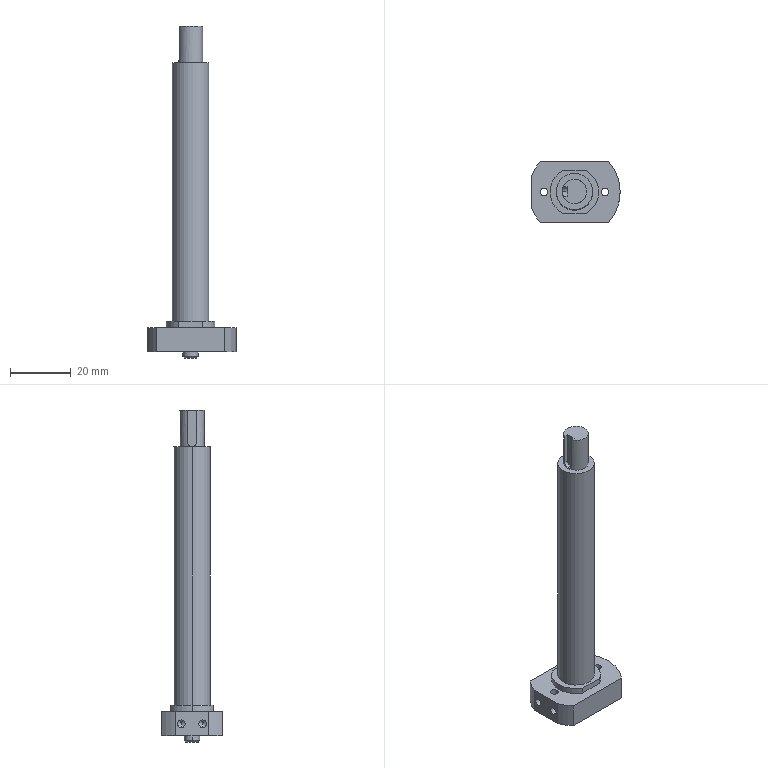Part | STEP file | 06-01-02 rotary shaft | 1 solid | 42 faces | box 29 x 20 x 109 mm | volume 14786 mm3 | cylinder 22 | plane 14 | cone 6 | commonest cylinder face diameters 2.5 x8 16 x3 30 x3 3 x2 5 x2 8 x2
STEP:
#1=CARTESIAN_POINT('',(-6.5,-3.5,2.75));
#2=VERTEX_POINT('',#1);
#3=CARTESIAN_POINT('',(-6.5,-3.5,5.25));
#4=VERTEX_POINT('',#3);
#5=CARTESIAN_POINT('',(-6.5,-3.5,4.));
#6=DIRECTION('',(-1.,0.,0.));
#7=DIRECTION('',(0.,0.,1.));
#8=AXIS2_PLACEMENT_3D('',#5,#6,#7);
#9=CIRCLE('',#8,1.25);
#10=EDGE_CURVE('',#2,#4,#9,.T.);
#11=ORIENTED_EDGE('',*,*,#10,.F.);
#12=CARTESIAN_POINT('',(-14.,-3.5,2.75));
#13=VERTEX_POINT('',#12);
#14=CARTESIAN_POINT('',(-14.,-3.5,2.75));
#15=DIRECTION('',(-1.,0.,0.));
#16=VECTOR('',#15,1000.);
#17=LINE('',#14,#16);
#18=EDGE_CURVE('',#2,#13,#17,.T.);
#19=ORIENTED_EDGE('',*,*,#18,.T.);
#20=CARTESIAN_POINT('',(-14.,-3.5,5.25));
#21=VERTEX_POINT('',#20);
#22=CARTESIAN_POINT('',(-14.,-3.5,4.));
#23=DIRECTION('',(-1.,0.,0.));
#24=DIRECTION('',(0.,0.,1.));
#25=AXIS2_PLACEMENT_3D('',#22,#23,#24);
#26=CIRCLE('',#25,1.25);
#27=EDGE_CURVE('',#13,#21,#26,.T.);
#28=ORIENTED_EDGE('',*,*,#27,.T.);
#29=CARTESIAN_POINT('',(-14.,-3.5,5.25));
#30=DIRECTION('',(-1.,0.,0.));
#31=VECTOR('',#30,1000.);
#32=LINE('',#29,#31);
#33=EDGE_CURVE('',#4,#21,#32,.T.);
#34=ORIENTED_EDGE('',*,*,#33,.F.);
#35=EDGE_LOOP('',(#11,#19,#28,#34));
#36=FACE_OUTER_BOUND('',#35,.T.);
#37=CARTESIAN_POINT('',(-14.,-3.5,4.));
#38=DIRECTION('',(-1.,0.,0.));
#39=DIRECTION('',(0.,0.,1.));
#40=AXIS2_PLACEMENT_3D('',#37,#38,#39);
#41=CYLINDRICAL_SURFACE('',#40,1.25);
#42=ADVANCED_FACE('',(#36),#41,.F.);
#43=CARTESIAN_POINT('',(-5.749,-3.5,4.));
#44=VERTEX_POINT('',#43);
#45=CARTESIAN_POINT('',(-6.5,-3.5,5.25));
#46=DIRECTION('',(-0.515,0.,0.8572));
#47=VECTOR('',#46,1000.);
#48=LINE('',#45,#47);
#49=EDGE_CURVE('',#44,#4,#48,.T.);
#50=ORIENTED_EDGE('',*,*,#49,.F.);
#51=CARTESIAN_POINT('',(-6.5,-3.5,2.75));
#52=DIRECTION('',(-0.515,0.,-0.8572));
#53=VECTOR('',#52,1000.);
#54=LINE('',#51,#53);
#55=EDGE_CURVE('',#44,#2,#54,.T.);
#56=ORIENTED_EDGE('',*,*,#55,.T.);
#57=ORIENTED_EDGE('',*,*,#10,.T.);
#58=EDGE_LOOP('',(#50,#56,#57));
#59=FACE_OUTER_BOUND('',#58,.T.);
#60=CARTESIAN_POINT('',(-6.5,-3.5,4.));
#61=DIRECTION('',(-1.,0.,0.));
#62=DIRECTION('',(0.,0.,1.));
#63=AXIS2_PLACEMENT_3D('',#60,#61,#62);
#64=CONICAL_SURFACE('',#63,1.25,1.03);
#65=ADVANCED_FACE('',(#59),#64,.F.);
#66=CARTESIAN_POINT('',(-6.5,3.5,2.75));
#67=VERTEX_POINT('',#66);
#68=CARTESIAN_POINT('',(-6.5,3.5,5.25));
#69=VERTEX_POINT('',#68);
#70=CARTESIAN_POINT('',(-6.5,3.5,4.));
#71=DIRECTION('',(-1.,0.,0.));
#72=DIRECTION('',(0.,0.,1.));
#73=AXIS2_PLACEMENT_3D('',#70,#71,#72);
#74=CIRCLE('',#73,1.25);
#75=EDGE_CURVE('',#67,#69,#74,.T.);
#76=ORIENTED_EDGE('',*,*,#75,.F.);
#77=CARTESIAN_POINT('',(-14.,3.5,2.75));
#78=VERTEX_POINT('',#77);
#79=CARTESIAN_POINT('',(-14.,3.5,2.75));
#80=DIRECTION('',(-1.,0.,0.));
#81=VECTOR('',#80,1000.);
#82=LINE('',#79,#81);
#83=EDGE_CURVE('',#67,#78,#82,.T.);
#84=ORIENTED_EDGE('',*,*,#83,.T.);
#85=CARTESIAN_POINT('',(-14.,3.5,5.25));
#86=VERTEX_POINT('',#85);
#87=CARTESIAN_POINT('',(-14.,3.5,4.));
#88=DIRECTION('',(-1.,0.,0.));
#89=DIRECTION('',(0.,0.,1.));
#90=AXIS2_PLACEMENT_3D('',#87,#88,#89);
#91=CIRCLE('',#90,1.25);
#92=EDGE_CURVE('',#78,#86,#91,.T.);
#93=ORIENTED_EDGE('',*,*,#92,.T.);
#94=CARTESIAN_POINT('',(-14.,3.5,5.25));
#95=DIRECTION('',(-1.,0.,0.));
#96=VECTOR('',#95,1000.);
#97=LINE('',#94,#96);
#98=EDGE_CURVE('',#69,#86,#97,.T.);
#99=ORIENTED_EDGE('',*,*,#98,.F.);
#100=EDGE_LOOP('',(#76,#84,#93,#99));
#101=FACE_OUTER_BOUND('',#100,.T.);
#102=CARTESIAN_POINT('',(-14.,3.5,4.));
#103=DIRECTION('',(-1.,0.,0.));
#104=DIRECTION('',(0.,0.,1.));
#105=AXIS2_PLACEMENT_3D('',#102,#103,#104);
#106=CYLINDRICAL_SURFACE('',#105,1.25);
#107=ADVANCED_FACE('',(#101),#106,.F.);
#108=CARTESIAN_POINT('',(-5.749,3.5,4.));
#109=VERTEX_POINT('',#108);
#110=CARTESIAN_POINT('',(-6.5,3.5,5.25));
#111=DIRECTION('',(-0.515,0.,0.8572));
#112=VECTOR('',#111,1000.);
#113=LINE('',#110,#112);
#114=EDGE_CURVE('',#109,#69,#113,.T.);
#115=ORIENTED_EDGE('',*,*,#114,.F.);
#116=CARTESIAN_POINT('',(-6.5,3.5,2.75));
#117=DIRECTION('',(-0.515,0.,-0.8572));
#118=VECTOR('',#117,1000.);
#119=LINE('',#116,#118);
#120=EDGE_CURVE('',#109,#67,#119,.T.);
#121=ORIENTED_EDGE('',*,*,#120,.T.);
#122=ORIENTED_EDGE('',*,*,#75,.T.);
#123=EDGE_LOOP('',(#115,#121,#122));
#124=FACE_OUTER_BOUND('',#123,.T.);
#125=CARTESIAN_POINT('',(-6.5,3.5,4.));
#126=DIRECTION('',(-1.,0.,0.));
#127=DIRECTION('',(0.,0.,1.));
#128=AXIS2_PLACEMENT_3D('',#125,#126,#127);
#129=CONICAL_SURFACE('',#128,1.25,1.03);
#130=ADVANCED_FACE('',(#124),#129,.F.);
#131=CARTESIAN_POINT('',(-2.,0.,-2.));
#132=VERTEX_POINT('',#131);
#133=CARTESIAN_POINT('',(2.,0.,-2.));
#134=VERTEX_POINT('',#133);
#135=CARTESIAN_POINT('',(0.,0.,-2.));
#136=DIRECTION('',(0.,0.,-1.));
#137=DIRECTION('',(-1.,0.,0.));
#138=AXIS2_PLACEMENT_3D('',#135,#136,#137);
#139=CIRCLE('',#138,2.);
#140=EDGE_CURVE('',#132,#134,#139,.T.);
#141=ORIENTED_EDGE('',*,*,#140,.F.);
#142=CARTESIAN_POINT('',(-2.5,0.,-1.5));
#143=VERTEX_POINT('',#142);
#144=CARTESIAN_POINT('',(-2.,0.,-2.));
#145=DIRECTION('',(-0.7071,0.,0.7071));
#146=VECTOR('',#145,1000.);
#147=LINE('',#144,#146);
#148=EDGE_CURVE('',#132,#143,#147,.T.);
#149=ORIENTED_EDGE('',*,*,#148,.T.);
#150=CARTESIAN_POINT('',(2.5,0.,-1.5));
#151=VERTEX_POINT('',#150);
#152=CARTESIAN_POINT('',(0.,0.,-1.5));
#153=DIRECTION('',(0.,0.,1.));
#154=DIRECTION('',(-1.,0.,0.));
#155=AXIS2_PLACEMENT_3D('',#152,#153,#154);
#156=CIRCLE('',#155,2.5);
#157=EDGE_CURVE('',#151,#143,#156,.T.);
#158=ORIENTED_EDGE('',*,*,#157,.F.);
#159=CARTESIAN_POINT('',(2.,0.,-2.));
#160=DIRECTION('',(0.7071,0.,0.7071));
#161=VECTOR('',#160,1000.);
#162=LINE('',#159,#161);
#163=EDGE_CURVE('',#134,#151,#162,.T.);
#164=ORIENTED_EDGE('',*,*,#163,.F.);
#165=EDGE_LOOP('',(#141,#149,#158,#164));
#166=FACE_OUTER_BOUND('',#165,.T.);
#167=CARTESIAN_POINT('',(0.,0.,-2.));
#168=DIRECTION('',(0.,0.,1.));
#169=DIRECTION('',(1.,0.,0.));
#170=AXIS2_PLACEMENT_3D('',#167,#168,#169);
#171=CONICAL_SURFACE('',#170,2.,0.7854);
#172=ADVANCED_FACE('',(#166),#171,.T.);
#173=CARTESIAN_POINT('',(8.75,0.,8.));
#174=VERTEX_POINT('',#173);
#175=CARTESIAN_POINT('',(11.25,0.,8.));
#176=VERTEX_POINT('',#175);
#177=CARTESIAN_POINT('',(10.,0.,8.));
#178=DIRECTION('',(0.,0.,1.));
#179=DIRECTION('',(1.,0.,0.));
#180=AXIS2_PLACEMENT_3D('',#177,#178,#179);
#181=CIRCLE('',#180,1.25);
#182=EDGE_CURVE('',#174,#176,#181,.T.);
#183=ORIENTED_EDGE('',*,*,#182,.T.);
#184=CARTESIAN_POINT('',(11.25,0.,0.));
#185=VERTEX_POINT('',#184);
#186=CARTESIAN_POINT('',(11.25,0.,0.));
#187=DIRECTION('',(0.,0.,-1.));
#188=VECTOR('',#187,1000.);
#189=LINE('',#186,#188);
#190=EDGE_CURVE('',#176,#185,#189,.T.);
#191=ORIENTED_EDGE('',*,*,#190,.T.);
#192=CARTESIAN_POINT('',(8.75,0.,0.));
#193=VERTEX_POINT('',#192);
#194=CARTESIAN_POINT('',(10.,0.,0.));
#195=DIRECTION('',(0.,0.,-1.));
#196=DIRECTION('',(-1.,0.,0.));
#197=AXIS2_PLACEMENT_3D('',#194,#195,#196);
#198=CIRCLE('',#197,1.25);
#199=EDGE_CURVE('',#185,#193,#198,.T.);
#200=ORIENTED_EDGE('',*,*,#199,.T.);
#201=CARTESIAN_POINT('',(8.75,0.,0.));
#202=DIRECTION('',(0.,0.,-1.));
#203=VECTOR('',#202,1000.);
#204=LINE('',#201,#203);
#205=EDGE_CURVE('',#174,#193,#204,.T.);
#206=ORIENTED_EDGE('',*,*,#205,.F.);
#207=EDGE_LOOP('',(#183,#191,#200,#206));
#208=FACE_OUTER_BOUND('',#207,.T.);
#209=CARTESIAN_POINT('',(10.,0.,0.));
#210=DIRECTION('',(0.,0.,-1.));
#211=DIRECTION('',(-1.,0.,0.));
#212=AXIS2_PLACEMENT_3D('',#209,#210,#211);
#213=CYLINDRICAL_SURFACE('',#212,1.25);
#214=ADVANCED_FACE('',(#208),#213,.F.);
#215=CARTESIAN_POINT('',(-11.25,0.,8.));
#216=VERTEX_POINT('',#215);
#217=CARTESIAN_POINT('',(-8.75,0.,8.));
#218=VERTEX_POINT('',#217);
#219=CARTESIAN_POINT('',(-10.,0.,8.));
#220=DIRECTION('',(0.,0.,1.));
#221=DIRECTION('',(1.,0.,0.));
#222=AXIS2_PLACEMENT_3D('',#219,#220,#221);
#223=CIRCLE('',#222,1.25);
#224=EDGE_CURVE('',#216,#218,#223,.T.);
#225=ORIENTED_EDGE('',*,*,#224,.T.);
#226=CARTESIAN_POINT('',(-8.75,0.,0.));
#227=VERTEX_POINT('',#226);
#228=CARTESIAN_POINT('',(-8.75,0.,0.));
#229=DIRECTION('',(0.,0.,-1.));
#230=VECTOR('',#229,1000.);
#231=LINE('',#228,#230);
#232=EDGE_CURVE('',#218,#227,#231,.T.);
#233=ORIENTED_EDGE('',*,*,#232,.T.);
#234=CARTESIAN_POINT('',(-11.25,0.,0.));
#235=VERTEX_POINT('',#234);
#236=CARTESIAN_POINT('',(-10.,0.,0.));
#237=DIRECTION('',(0.,0.,-1.));
#238=DIRECTION('',(-1.,0.,0.));
#239=AXIS2_PLACEMENT_3D('',#236,#237,#238);
#240=CIRCLE('',#239,1.25);
#241=EDGE_CURVE('',#227,#235,#240,.T.);
#242=ORIENTED_EDGE('',*,*,#241,.T.);
#243=CARTESIAN_POINT('',(-11.25,0.,0.));
#244=DIRECTION('',(0.,0.,-1.));
#245=VECTOR('',#244,1000.);
#246=LINE('',#243,#245);
#247=EDGE_CURVE('',#216,#235,#246,.T.);
#248=ORIENTED_EDGE('',*,*,#247,.F.);
#249=EDGE_LOOP('',(#225,#233,#242,#248));
#250=FACE_OUTER_BOUND('',#249,.T.);
#251=CARTESIAN_POINT('',(-10.,0.,0.));
#252=DIRECTION('',(0.,0.,-1.));
#253=DIRECTION('',(-1.,0.,0.));
#254=AXIS2_PLACEMENT_3D('',#251,#252,#253);
#255=CYLINDRICAL_SURFACE('',#254,1.25);
#256=ADVANCED_FACE('',(#250),#255,.F.);
#257=CARTESIAN_POINT('',(4.,0.,107.));
#258=VERTEX_POINT('',#257);
#259=CARTESIAN_POINT('',(-3.708,1.5,107.));
#260=VERTEX_POINT('',#259);
#261=CARTESIAN_POINT('',(0.,0.,107.));
#262=DIRECTION('',(0.,0.,1.));
#263=DIRECTION('',(1.,0.,0.));
#264=AXIS2_PLACEMENT_3D('',#261,#262,#263);
#265=CIRCLE('',#264,4.);
#266=EDGE_CURVE('',#258,#260,#265,.T.);
#267=ORIENTED_EDGE('',*,*,#266,.F.);
#268=CARTESIAN_POINT('',(4.,0.,95.));
#269=VERTEX_POINT('',#268);
#270=CARTESIAN_POINT('',(4.,0.,107.));
#271=DIRECTION('',(0.,0.,-1.));
#272=VECTOR('',#271,1000.);
#273=LINE('',#270,#272);
#274=EDGE_CURVE('',#258,#269,#273,.T.);
#275=ORIENTED_EDGE('',*,*,#274,.T.);
#276=CARTESIAN_POINT('',(-4.,0.,95.));
#277=VERTEX_POINT('',#276);
#278=CARTESIAN_POINT('',(0.,0.,95.));
#279=DIRECTION('',(0.,0.,1.));
#280=DIRECTION('',(1.,0.,0.));
#281=AXIS2_PLACEMENT_3D('',#278,#279,#280);
#282=CIRCLE('',#281,4.);
#283=EDGE_CURVE('',#269,#277,#282,.T.);
#284=ORIENTED_EDGE('',*,*,#283,.T.);
#285=CARTESIAN_POINT('',(-3.708,1.5,96.5));
#286=VERTEX_POINT('',#285);
#287=CARTESIAN_POINT('',(-4.,0.,95.));
#288=CARTESIAN_POINT('',(-4.,0.1,95.));
#289=CARTESIAN_POINT('',(-3.996,0.1982,95.01));
#290=CARTESIAN_POINT('',(-3.982,0.3911,95.049));
#291=CARTESIAN_POINT('',(-3.971,0.4868,95.078));
#292=CARTESIAN_POINT('',(-3.932,0.7587,95.191));
#293=CARTESIAN_POINT('',(-3.894,0.9238,95.302));
#294=CARTESIAN_POINT('',(-3.819,1.198,95.576));
#295=CARTESIAN_POINT('',(-3.781,1.309,95.742));
#296=CARTESIAN_POINT('',(-3.725,1.459,96.102));
#297=CARTESIAN_POINT('',(-3.708,1.5,96.3));
#298=CARTESIAN_POINT('',(-3.708,1.5,96.5));
#299=B_SPLINE_CURVE_WITH_KNOTS('',3,(#287,#288,#289,#290,#291,#292,#293,#294,#295,#296,#297,#298),.UNSPECIFIED.,.F.,.F.,(4,2,2,2,2,4),(0.,0.0002957,0.0005913,0.001183,0.001774,0.002365),.UNSPECIFIED.);
#300=EDGE_CURVE('',#277,#286,#299,.T.);
#301=ORIENTED_EDGE('',*,*,#300,.T.);
#302=CARTESIAN_POINT('',(-3.708,1.5,107.));
#303=DIRECTION('',(0.,0.,1.));
#304=VECTOR('',#303,1000.);
#305=LINE('',#302,#304);
#306=EDGE_CURVE('',#286,#260,#305,.T.);
#307=ORIENTED_EDGE('',*,*,#306,.T.);
#308=EDGE_LOOP('',(#267,#275,#284,#301,#307));
#309=FACE_OUTER_BOUND('',#308,.T.);
#310=CARTESIAN_POINT('',(0.,0.,107.));
#311=DIRECTION('',(0.,0.,-1.));
#312=DIRECTION('',(-1.,0.,0.));
#313=AXIS2_PLACEMENT_3D('',#310,#311,#312);
#314=CYLINDRICAL_SURFACE('',#313,4.);
#315=ADVANCED_FACE('',(#309),#314,.T.);
#316=CARTESIAN_POINT('',(6.,0.,95.));
#317=VERTEX_POINT('',#316);
#318=CARTESIAN_POINT('',(-6.,0.,95.));
#319=VERTEX_POINT('',#318);
#320=CARTESIAN_POINT('',(0.,0.,95.));
#321=DIRECTION('',(0.,0.,1.));
#322=DIRECTION('',(1.,0.,0.));
#323=AXIS2_PLACEMENT_3D('',#320,#321,#322);
#324=CIRCLE('',#323,6.);
#325=EDGE_CURVE('',#317,#319,#324,.T.);
#326=ORIENTED_EDGE('',*,*,#325,.F.);
#327=CARTESIAN_POINT('',(6.,0.,10.));
#328=VERTEX_POINT('',#327);
#329=CARTESIAN_POINT('',(6.,0.,95.));
#330=DIRECTION('',(0.,0.,-1.));
#331=VECTOR('',#330,1000.);
#332=LINE('',#329,#331);
#333=EDGE_CURVE('',#317,#328,#332,.T.);
#334=ORIENTED_EDGE('',*,*,#333,.T.);
#335=CARTESIAN_POINT('',(-6.,0.,10.));
#336=VERTEX_POINT('',#335);
#337=CARTESIAN_POINT('',(0.,0.,10.));
#338=DIRECTION('',(0.,0.,1.));
#339=DIRECTION('',(1.,0.,0.));
#340=AXIS2_PLACEMENT_3D('',#337,#338,#339);
#341=CIRCLE('',#340,6.);
#342=EDGE_CURVE('',#328,#336,#341,.T.);
#343=ORIENTED_EDGE('',*,*,#342,.T.);
#344=CARTESIAN_POINT('',(-6.,0.,95.));
#345=DIRECTION('',(0.,0.,-1.));
#346=VECTOR('',#345,1000.);
#347=LINE('',#344,#346);
#348=EDGE_CURVE('',#319,#336,#347,.T.);
#349=ORIENTED_EDGE('',*,*,#348,.F.);
#350=EDGE_LOOP('',(#326,#334,#343,#349));
#351=FACE_OUTER_BOUND('',#350,.T.);
#352=CARTESIAN_POINT('',(0.,0.,95.));
#353=DIRECTION('',(0.,0.,-1.));
#354=DIRECTION('',(-1.,0.,0.));
#355=AXIS2_PLACEMENT_3D('',#352,#353,#354);
#356=CYLINDRICAL_SURFACE('',#355,6.);
#357=ADVANCED_FACE('',(#351),#356,.T.);
#358=CARTESIAN_POINT('',(-8.,0.,10.));
#359=VERTEX_POINT('',#358);
#360=CARTESIAN_POINT('',(-3.873,-7.,10.));
#361=VERTEX_POINT('',#360);
#362=CARTESIAN_POINT('',(0.,0.,10.));
#363=DIRECTION('',(0.,0.,1.));
#364=DIRECTION('',(1.,0.,0.));
#365=AXIS2_PLACEMENT_3D('',#362,#363,#364);
#366=CIRCLE('',#365,8.);
#367=EDGE_CURVE('',#359,#361,#366,.T.);
#368=ORIENTED_EDGE('',*,*,#367,.F.);
#369=CARTESIAN_POINT('',(-8.,0.,8.));
#370=VERTEX_POINT('',#369);
#371=CARTESIAN_POINT('',(-8.,0.,10.));
#372=DIRECTION('',(0.,0.,-1.));
#373=VECTOR('',#372,1000.);
#374=LINE('',#371,#373);
#375=EDGE_CURVE('',#359,#370,#374,.T.);
#376=ORIENTED_EDGE('',*,*,#375,.T.);
#377=CARTESIAN_POINT('',(-3.873,-7.,8.));
#378=VERTEX_POINT('',#377);
#379=CARTESIAN_POINT('',(0.,0.,8.));
#380=DIRECTION('',(0.,0.,1.));
#381=DIRECTION('',(1.,0.,0.));
#382=AXIS2_PLACEMENT_3D('',#379,#380,#381);
#383=CIRCLE('',#382,8.);
#384=EDGE_CURVE('',#370,#378,#383,.T.);
#385=ORIENTED_EDGE('',*,*,#384,.T.);
#386=CARTESIAN_POINT('',(-3.873,-7.,10.));
#387=DIRECTION('',(0.,0.,-1.));
#388=VECTOR('',#387,1000.);
#389=LINE('',#386,#388);
#390=EDGE_CURVE('',#361,#378,#389,.T.);
#391=ORIENTED_EDGE('',*,*,#390,.F.);
#392=EDGE_LOOP('',(#368,#376,#385,#391));
#393=FACE_OUTER_BOUND('',#392,.T.);
#394=CARTESIAN_POINT('',(0.,0.,10.));
#395=DIRECTION('',(0.,0.,-1.));
#396=DIRECTION('',(-1.,0.,0.));
#397=AXIS2_PLACEMENT_3D('',#394,#395,#396);
#398=CYLINDRICAL_SURFACE('',#397,8.);
#399=ADVANCED_FACE('',(#393),#398,.T.);
#400=ORIENTED_EDGE('',*,*,#157,.T.);
#401=CARTESIAN_POINT('',(-2.5,0.,0.));
#402=VERTEX_POINT('',#401);
#403=CARTESIAN_POINT('',(-2.5,0.,-2.));
#404=DIRECTION('',(0.,0.,1.));
#405=VECTOR('',#404,1000.);
#406=LINE('',#403,#405);
#407=EDGE_CURVE('',#143,#402,#406,.T.);
#408=ORIENTED_EDGE('',*,*,#407,.T.);
#409=CARTESIAN_POINT('',(2.5,0.,0.));
#410=VERTEX_POINT('',#409);
#411=CARTESIAN_POINT('',(0.,0.,0.));
#412=DIRECTION('',(0.,0.,-1.));
#413=DIRECTION('',(1.,0.,0.));
#414=AXIS2_PLACEMENT_3D('',#411,#412,#413);
#415=CIRCLE('',#414,2.5);
#416=EDGE_CURVE('',#402,#410,#415,.T.);
#417=ORIENTED_EDGE('',*,*,#416,.T.);
#418=CARTESIAN_POINT('',(2.5,0.,-2.));
#419=DIRECTION('',(0.,0.,1.));
#420=VECTOR('',#419,1000.);
#421=LINE('',#418,#420);
#422=EDGE_CURVE('',#151,#410,#421,.T.);
#423=ORIENTED_EDGE('',*,*,#422,.F.);
#424=EDGE_LOOP('',(#400,#408,#417,#423));
#425=FACE_OUTER_BOUND('',#424,.T.);
#426=CARTESIAN_POINT('',(0.,0.,-2.));
#427=DIRECTION('',(0.,0.,1.));
#428=DIRECTION('',(1.,0.,0.));
#429=AXIS2_PLACEMENT_3D('',#426,#427,#428);
#430=CYLINDRICAL_SURFACE('',#429,2.5);
#431=ADVANCED_FACE('',(#425),#430,.T.);
#432=CARTESIAN_POINT('',(-14.,-5.385,0.));
#433=VERTEX_POINT('',#432);
#434=CARTESIAN_POINT('',(-14.,-5.385,8.));
#435=VERTEX_POINT('',#434);
#436=CARTESIAN_POINT('',(-14.,-5.385,17.));
#437=DIRECTION('',(0.,0.,1.));
#438=VECTOR('',#437,1000.);
#439=LINE('',#436,#438);
#440=EDGE_CURVE('',#433,#435,#439,.T.);
#441=ORIENTED_EDGE('',*,*,#440,.F.);
#442=CARTESIAN_POINT('',(-11.18,-10.,0.));
#443=VERTEX_POINT('',#442);
#444=CARTESIAN_POINT('',(0.,0.,0.));
#445=DIRECTION('',(0.,0.,-1.));
#446=DIRECTION('',(-1.,0.,0.));
#447=AXIS2_PLACEMENT_3D('',#444,#445,#446);
#448=CIRCLE('',#447,15.);
#449=EDGE_CURVE('',#443,#433,#448,.T.);
#450=ORIENTED_EDGE('',*,*,#449,.F.);
#451=CARTESIAN_POINT('',(-11.18,-10.,8.));
#452=VERTEX_POINT('',#451);
#453=CARTESIAN_POINT('',(-11.18,-10.,17.));
#454=DIRECTION('',(0.,0.,1.));
#455=VECTOR('',#454,1000.);
#456=LINE('',#453,#455);
#457=EDGE_CURVE('',#443,#452,#456,.T.);
#458=ORIENTED_EDGE('',*,*,#457,.T.);
#459=CARTESIAN_POINT('',(0.,0.,8.));
#460=DIRECTION('',(0.,0.,1.));
#461=DIRECTION('',(1.,0.,0.));
#462=AXIS2_PLACEMENT_3D('',#459,#460,#461);
#463=CIRCLE('',#462,15.);
#464=EDGE_CURVE('',#435,#452,#463,.T.);
#465=ORIENTED_EDGE('',*,*,#464,.F.);
#466=EDGE_LOOP('',(#441,#450,#458,#465));
#467=FACE_OUTER_BOUND('',#466,.T.);
#468=CARTESIAN_POINT('',(0.,0.,17.));
#469=DIRECTION('',(0.,0.,-1.));
#470=DIRECTION('',(-1.,0.,0.));
#471=AXIS2_PLACEMENT_3D('',#468,#469,#470);
#472=CYLINDRICAL_SURFACE('',#471,15.);
#473=ADVANCED_FACE('',(#467),#472,.T.);
#474=CARTESIAN_POINT('',(0.,0.,95.));
#475=DIRECTION('',(0.,0.,1.));
#476=DIRECTION('',(1.,0.,0.));
#477=AXIS2_PLACEMENT_3D('',#474,#475,#476);
#478=CIRCLE('',#477,4.);
#479=EDGE_CURVE('',#277,#269,#478,.T.);
#480=ORIENTED_EDGE('',*,*,#479,.F.);
#481=ORIENTED_EDGE('',*,*,#283,.F.);
#482=EDGE_LOOP('',(#480,#481));
#483=FACE_BOUND('',#482,.T.);
#484=CARTESIAN_POINT('',(0.,0.,95.));
#485=DIRECTION('',(0.,0.,1.));
#486=DIRECTION('',(1.,0.,0.));
#487=AXIS2_PLACEMENT_3D('',#484,#485,#486);
#488=CIRCLE('',#487,6.);
#489=EDGE_CURVE('',#319,#317,#488,.T.);
#490=ORIENTED_EDGE('',*,*,#489,.T.);
#491=ORIENTED_EDGE('',*,*,#325,.T.);
#492=EDGE_LOOP('',(#490,#491));
#493=FACE_OUTER_BOUND('',#492,.T.);
#494=CARTESIAN_POINT('',(0.,0.,95.));
#495=DIRECTION('',(0.,0.,1.));
#496=DIRECTION('',(1.,0.,0.));
#497=AXIS2_PLACEMENT_3D('',#494,#495,#496);
#498=PLANE('',#497);
#499=ADVANCED_FACE('',(#483,#493),#498,.T.);
#500=CARTESIAN_POINT('',(3.873,-7.,10.));
#501=VERTEX_POINT('',#500);
#502=CARTESIAN_POINT('',(3.873,7.,10.));
#503=VERTEX_POINT('',#502);
#504=CARTESIAN_POINT('',(0.,0.,10.));
#505=DIRECTION('',(0.,0.,1.));
#506=DIRECTION('',(1.,0.,0.));
#507=AXIS2_PLACEMENT_3D('',#504,#505,#506);
#508=CIRCLE('',#507,8.);
#509=EDGE_CURVE('',#501,#503,#508,.T.);
#510=ORIENTED_EDGE('',*,*,#509,.T.);
#511=CARTESIAN_POINT('',(-3.873,7.,10.));
#512=VERTEX_POINT('',#511);
#513=CARTESIAN_POINT('',(-3.873,7.,10.));
#514=DIRECTION('',(-1.,0.,0.));
#515=VECTOR('',#514,1000.);
#516=LINE('',#513,#515);
#517=EDGE_CURVE('',#503,#512,#516,.T.);
#518=ORIENTED_EDGE('',*,*,#517,.T.);
#519=CARTESIAN_POINT('',(0.,0.,10.));
#520=DIRECTION('',(0.,0.,1.));
#521=DIRECTION('',(1.,0.,0.));
#522=AXIS2_PLACEMENT_3D('',#519,#520,#521);
#523=CIRCLE('',#522,8.);
#524=EDGE_CURVE('',#512,#359,#523,.T.);
#525=ORIENTED_EDGE('',*,*,#524,.T.);
#526=ORIENTED_EDGE('',*,*,#367,.T.);
#527=CARTESIAN_POINT('',(-3.873,-7.,10.));
#528=DIRECTION('',(1.,0.,0.));
#529=VECTOR('',#528,1000.);
#530=LINE('',#527,#529);
#531=EDGE_CURVE('',#361,#501,#530,.T.);
#532=ORIENTED_EDGE('',*,*,#531,.T.);
#533=EDGE_LOOP('',(#510,#518,#525,#526,#532));
#534=FACE_OUTER_BOUND('',#533,.T.);
#535=CARTESIAN_POINT('',(0.,0.,10.));
#536=DIRECTION('',(0.,0.,1.));
#537=DIRECTION('',(1.,0.,0.));
#538=AXIS2_PLACEMENT_3D('',#535,#536,#537);
#539=CIRCLE('',#538,6.);
#540=EDGE_CURVE('',#336,#328,#539,.T.);
#541=ORIENTED_EDGE('',*,*,#540,.F.);
#542=ORIENTED_EDGE('',*,*,#342,.F.);
#543=EDGE_LOOP('',(#541,#542));
#544=FACE_BOUND('',#543,.T.);
#545=CARTESIAN_POINT('',(0.,0.,10.));
#546=DIRECTION('',(0.,0.,1.));
#547=DIRECTION('',(1.,0.,0.));
#548=AXIS2_PLACEMENT_3D('',#545,#546,#547);
#549=PLANE('',#548);
#550=ADVANCED_FACE('',(#534,#544),#549,.T.);
#551=CARTESIAN_POINT('',(-14.,5.385,8.));
#552=VERTEX_POINT('',#551);
#553=CARTESIAN_POINT('',(-14.,-10.,8.));
#554=DIRECTION('',(0.,1.,0.));
#555=VECTOR('',#554,1000.);
#556=LINE('',#553,#555);
#557=EDGE_CURVE('',#435,#552,#556,.T.);
#558=ORIENTED_EDGE('',*,*,#557,.F.);
#559=ORIENTED_EDGE('',*,*,#464,.T.);
#560=CARTESIAN_POINT('',(11.18,-10.,8.));
#561=VERTEX_POINT('',#560);
#562=CARTESIAN_POINT('',(-15.,-10.,8.));
#563=DIRECTION('',(1.,0.,0.));
#564=VECTOR('',#563,1000.);
#565=LINE('',#562,#564);
#566=EDGE_CURVE('',#452,#561,#565,.T.);
#567=ORIENTED_EDGE('',*,*,#566,.T.);
#568=CARTESIAN_POINT('',(11.18,10.,8.));
#569=VERTEX_POINT('',#568);
#570=CARTESIAN_POINT('',(0.,0.,8.));
#571=DIRECTION('',(0.,0.,1.));
#572=DIRECTION('',(1.,0.,0.));
#573=AXIS2_PLACEMENT_3D('',#570,#571,#572);
#574=CIRCLE('',#573,15.);
#575=EDGE_CURVE('',#561,#569,#574,.T.);
#576=ORIENTED_EDGE('',*,*,#575,.T.);
#577=CARTESIAN_POINT('',(-11.18,10.,8.));
#578=VERTEX_POINT('',#577);
#579=CARTESIAN_POINT('',(-15.,10.,8.));
#580=DIRECTION('',(-1.,0.,0.));
#581=VECTOR('',#580,1000.);
#582=LINE('',#579,#581);
#583=EDGE_CURVE('',#569,#578,#582,.T.);
#584=ORIENTED_EDGE('',*,*,#583,.T.);
#585=CARTESIAN_POINT('',(0.,0.,8.));
#586=DIRECTION('',(0.,0.,1.));
#587=DIRECTION('',(1.,0.,0.));
#588=AXIS2_PLACEMENT_3D('',#585,#586,#587);
#589=CIRCLE('',#588,15.);
#590=EDGE_CURVE('',#578,#552,#589,.T.);
#591=ORIENTED_EDGE('',*,*,#590,.T.);
#592=EDGE_LOOP('',(#558,#559,#567,#576,#584,#591));
#593=FACE_OUTER_BOUND('',#592,.T.);
#594=ORIENTED_EDGE('',*,*,#182,.F.);
#595=CARTESIAN_POINT('',(10.,0.,8.));
#596=DIRECTION('',(0.,0.,1.));
#597=DIRECTION('',(1.,0.,0.));
#598=AXIS2_PLACEMENT_3D('',#595,#596,#597);
#599=CIRCLE('',#598,1.25);
#600=EDGE_CURVE('',#176,#174,#599,.T.);
#601=ORIENTED_EDGE('',*,*,#600,.F.);
#602=EDGE_LOOP('',(#594,#601));
#603=FACE_BOUND('',#602,.T.);
#604=ORIENTED_EDGE('',*,*,#224,.F.);
#605=CARTESIAN_POINT('',(-10.,0.,8.));
#606=DIRECTION('',(0.,0.,1.));
#607=DIRECTION('',(1.,0.,0.));
#608=AXIS2_PLACEMENT_3D('',#605,#606,#607);
#609=CIRCLE('',#608,1.25);
#610=EDGE_CURVE('',#218,#216,#609,.T.);
#611=ORIENTED_EDGE('',*,*,#610,.F.);
#612=EDGE_LOOP('',(#604,#611));
#613=FACE_BOUND('',#612,.T.);
#614=CARTESIAN_POINT('',(3.873,7.,8.));
#615=VERTEX_POINT('',#614);
#616=CARTESIAN_POINT('',(-3.873,7.,8.));
#617=VERTEX_POINT('',#616);
#618=CARTESIAN_POINT('',(-3.873,7.,8.));
#619=DIRECTION('',(-1.,0.,0.));
#620=VECTOR('',#619,1000.);
#621=LINE('',#618,#620);
#622=EDGE_CURVE('',#615,#617,#621,.T.);
#623=ORIENTED_EDGE('',*,*,#622,.F.);
#624=CARTESIAN_POINT('',(3.873,-7.,8.));
#625=VERTEX_POINT('',#624);
#626=CARTESIAN_POINT('',(0.,0.,8.));
#627=DIRECTION('',(0.,0.,1.));
#628=DIRECTION('',(1.,0.,0.));
#629=AXIS2_PLACEMENT_3D('',#626,#627,#628);
#630=CIRCLE('',#629,8.);
#631=EDGE_CURVE('',#625,#615,#630,.T.);
#632=ORIENTED_EDGE('',*,*,#631,.F.);
#633=CARTESIAN_POINT('',(-3.873,-7.,8.));
#634=DIRECTION('',(1.,0.,0.));
#635=VECTOR('',#634,1000.);
#636=LINE('',#633,#635);
#637=EDGE_CURVE('',#378,#625,#636,.T.);
#638=ORIENTED_EDGE('',*,*,#637,.F.);
#639=ORIENTED_EDGE('',*,*,#384,.F.);
#640=CARTESIAN_POINT('',(0.,0.,8.));
#641=DIRECTION('',(0.,0.,1.));
#642=DIRECTION('',(1.,0.,0.));
#643=AXIS2_PLACEMENT_3D('',#640,#641,#642);
#644=CIRCLE('',#643,8.);
#645=EDGE_CURVE('',#617,#370,#644,.T.);
#646=ORIENTED_EDGE('',*,*,#645,.F.);
#647=EDGE_LOOP('',(#623,#632,#638,#639,#646));
#648=FACE_BOUND('',#647,.T.);
#649=CARTESIAN_POINT('',(15.,-10.,8.));
#650=DIRECTION('',(0.,0.,1.));
#651=DIRECTION('',(1.,0.,0.));
#652=AXIS2_PLACEMENT_3D('',#649,#650,#651);
#653=PLANE('',#652);
#654=ADVANCED_FACE('',(#593,#603,#613,#648),#653,.T.);
#655=CARTESIAN_POINT('',(10.,0.,0.));
#656=DIRECTION('',(0.,0.,-1.));
#657=DIRECTION('',(-1.,0.,0.));
#658=AXIS2_PLACEMENT_3D('',#655,#656,#657);
#659=CIRCLE('',#658,1.25);
#660=EDGE_CURVE('',#193,#185,#659,.T.);
#661=ORIENTED_EDGE('',*,*,#660,.F.);
#662=ORIENTED_EDGE('',*,*,#199,.F.);
#663=EDGE_LOOP('',(#661,#662));
#664=FACE_BOUND('',#663,.T.);
#665=CARTESIAN_POINT('',(-10.,0.,0.));
#666=DIRECTION('',(0.,0.,-1.));
#667=DIRECTION('',(-1.,0.,0.));
#668=AXIS2_PLACEMENT_3D('',#665,#666,#667);
#669=CIRCLE('',#668,1.25);
#670=EDGE_CURVE('',#235,#227,#669,.T.);
#671=ORIENTED_EDGE('',*,*,#670,.F.);
#672=ORIENTED_EDGE('',*,*,#241,.F.);
#673=EDGE_LOOP('',(#671,#672));
#674=FACE_BOUND('',#673,.T.);
#675=CARTESIAN_POINT('',(0.,0.,0.));
#676=DIRECTION('',(0.,0.,-1.));
#677=DIRECTION('',(1.,0.,0.));
#678=AXIS2_PLACEMENT_3D('',#675,#676,#677);
#679=CIRCLE('',#678,2.5);
#680=EDGE_CURVE('',#410,#402,#679,.T.);
#681=ORIENTED_EDGE('',*,*,#680,.F.);
#682=ORIENTED_EDGE('',*,*,#416,.F.);
#683=EDGE_LOOP('',(#681,#682));
#684=FACE_BOUND('',#683,.T.);
#685=ORIENTED_EDGE('',*,*,#449,.T.);
#686=CARTESIAN_POINT('',(-14.,5.385,0.));
#687=VERTEX_POINT('',#686);
#688=CARTESIAN_POINT('',(-14.,8.088,0.));
#689=DIRECTION('',(0.,-1.,0.));
#690=VECTOR('',#689,1000.);
#691=LINE('',#688,#690);
#692=EDGE_CURVE('',#687,#433,#691,.T.);
#693=ORIENTED_EDGE('',*,*,#692,.F.);
#694=CARTESIAN_POINT('',(-11.18,10.,0.));
#695=VERTEX_POINT('',#694);
#696=CARTESIAN_POINT('',(0.,0.,0.));
#697=DIRECTION('',(0.,0.,-1.));
#698=DIRECTION('',(-1.,0.,0.));
#699=AXIS2_PLACEMENT_3D('',#696,#697,#698);
#700=CIRCLE('',#699,15.);
#701=EDGE_CURVE('',#687,#695,#700,.T.);
#702=ORIENTED_EDGE('',*,*,#701,.T.);
#703=CARTESIAN_POINT('',(11.18,10.,0.));
#704=VERTEX_POINT('',#703);
#705=CARTESIAN_POINT('',(-15.,10.,0.));
#706=DIRECTION('',(-1.,0.,0.));
#707=VECTOR('',#706,1000.);
#708=LINE('',#705,#707);
#709=EDGE_CURVE('',#704,#695,#708,.T.);
#710=ORIENTED_EDGE('',*,*,#709,.F.);
#711=CARTESIAN_POINT('',(11.18,-10.,0.));
#712=VERTEX_POINT('',#711);
#713=CARTESIAN_POINT('',(0.,0.,0.));
#714=DIRECTION('',(0.,0.,-1.));
#715=DIRECTION('',(-1.,0.,0.));
#716=AXIS2_PLACEMENT_3D('',#713,#714,#715);
#717=CIRCLE('',#716,15.);
#718=EDGE_CURVE('',#704,#712,#717,.T.);
#719=ORIENTED_EDGE('',*,*,#718,.T.);
#720=CARTESIAN_POINT('',(-15.,-10.,0.));
#721=DIRECTION('',(1.,0.,0.));
#722=VECTOR('',#721,1000.);
#723=LINE('',#720,#722);
#724=EDGE_CURVE('',#443,#712,#723,.T.);
#725=ORIENTED_EDGE('',*,*,#724,.F.);
#726=EDGE_LOOP('',(#685,#693,#702,#710,#719,#725));
#727=FACE_OUTER_BOUND('',#726,.T.);
#728=CARTESIAN_POINT('',(15.,-10.,0.));
#729=DIRECTION('',(0.,0.,1.));
#730=DIRECTION('',(1.,0.,0.));
#731=AXIS2_PLACEMENT_3D('',#728,#729,#730);
#732=PLANE('',#731);
#733=ADVANCED_FACE('',(#664,#674,#684,#727),#732,.F.);
#734=CARTESIAN_POINT('',(-11.18,10.,17.));
#735=DIRECTION('',(0.,0.,-1.));
#736=VECTOR('',#735,1000.);
#737=LINE('',#734,#736);
#738=EDGE_CURVE('',#578,#695,#737,.T.);
#739=ORIENTED_EDGE('',*,*,#738,.F.);
#740=ORIENTED_EDGE('',*,*,#583,.F.);
#741=CARTESIAN_POINT('',(11.18,10.,17.));
#742=DIRECTION('',(0.,0.,1.));
#743=VECTOR('',#742,1000.);
#744=LINE('',#741,#743);
#745=EDGE_CURVE('',#704,#569,#744,.T.);
#746=ORIENTED_EDGE('',*,*,#745,.F.);
#747=ORIENTED_EDGE('',*,*,#709,.T.);
#748=EDGE_LOOP('',(#739,#740,#746,#747));
#749=FACE_OUTER_BOUND('',#748,.T.);
#750=CARTESIAN_POINT('',(-15.,10.,8.));
#751=DIRECTION('',(0.,-1.,0.));
#752=DIRECTION('',(0.,0.,-1.));
#753=AXIS2_PLACEMENT_3D('',#750,#751,#752);
#754=PLANE('',#753);
#755=ADVANCED_FACE('',(#749),#754,.F.);
#756=CARTESIAN_POINT('',(11.18,-10.,17.));
#757=DIRECTION('',(0.,0.,-1.));
#758=VECTOR('',#757,1000.);
#759=LINE('',#756,#758);
#760=EDGE_CURVE('',#561,#712,#759,.T.);
#761=ORIENTED_EDGE('',*,*,#760,.F.);
#762=ORIENTED_EDGE('',*,*,#566,.F.);
#763=ORIENTED_EDGE('',*,*,#457,.F.);
#764=ORIENTED_EDGE('',*,*,#724,.T.);
#765=EDGE_LOOP('',(#761,#762,#763,#764));
#766=FACE_OUTER_BOUND('',#765,.T.);
#767=CARTESIAN_POINT('',(-15.,-10.,8.));
#768=DIRECTION('',(0.,1.,0.));
#769=DIRECTION('',(0.,0.,1.));
#770=AXIS2_PLACEMENT_3D('',#767,#768,#769);
#771=PLANE('',#770);
#772=ADVANCED_FACE('',(#766),#771,.F.);
#773=ORIENTED_EDGE('',*,*,#407,.F.);
#774=CARTESIAN_POINT('',(0.,0.,-1.5));
#775=DIRECTION('',(0.,0.,1.));
#776=DIRECTION('',(-1.,0.,0.));
#777=AXIS2_PLACEMENT_3D('',#774,#775,#776);
#778=CIRCLE('',#777,2.5);
#779=EDGE_CURVE('',#143,#151,#778,.T.);
#780=ORIENTED_EDGE('',*,*,#779,.T.);
#781=ORIENTED_EDGE('',*,*,#422,.T.);
#782=ORIENTED_EDGE('',*,*,#680,.T.);
#783=EDGE_LOOP('',(#773,#780,#781,#782));
#784=FACE_OUTER_BOUND('',#783,.T.);
#785=CARTESIAN_POINT('',(0.,0.,-2.));
#786=DIRECTION('',(0.,0.,1.));
#787=DIRECTION('',(1.,0.,0.));
#788=AXIS2_PLACEMENT_3D('',#785,#786,#787);
#789=CYLINDRICAL_SURFACE('',#788,2.5);
#790=ADVANCED_FACE('',(#784),#789,.T.);
#791=CARTESIAN_POINT('',(0.,0.,-2.));
#792=DIRECTION('',(0.,0.,-1.));
#793=DIRECTION('',(-1.,0.,0.));
#794=AXIS2_PLACEMENT_3D('',#791,#792,#793);
#795=CIRCLE('',#794,2.);
#796=EDGE_CURVE('',#134,#132,#795,.T.);
#797=ORIENTED_EDGE('',*,*,#796,.T.);
#798=ORIENTED_EDGE('',*,*,#140,.T.);
#799=EDGE_LOOP('',(#797,#798));
#800=FACE_OUTER_BOUND('',#799,.T.);
#801=CARTESIAN_POINT('',(0.,0.,-2.));
#802=DIRECTION('',(0.,0.,-1.));
#803=DIRECTION('',(-1.,0.,0.));
#804=AXIS2_PLACEMENT_3D('',#801,#802,#803);
#805=PLANE('',#804);
#806=ADVANCED_FACE('',(#800),#805,.T.);
#807=ORIENTED_EDGE('',*,*,#745,.T.);
#808=ORIENTED_EDGE('',*,*,#575,.F.);
#809=ORIENTED_EDGE('',*,*,#760,.T.);
#810=ORIENTED_EDGE('',*,*,#718,.F.);
#811=EDGE_LOOP('',(#807,#808,#809,#810));
#812=FACE_OUTER_BOUND('',#811,.T.);
#813=CARTESIAN_POINT('',(0.,0.,17.));
#814=DIRECTION('',(0.,0.,-1.));
#815=DIRECTION('',(-1.,0.,0.));
#816=AXIS2_PLACEMENT_3D('',#813,#814,#815);
#817=CYLINDRICAL_SURFACE('',#816,15.);
#818=ADVANCED_FACE('',(#812),#817,.T.);
#819=CARTESIAN_POINT('',(-14.,5.385,17.));
#820=DIRECTION('',(0.,0.,-1.));
#821=VECTOR('',#820,1000.);
#822=LINE('',#819,#821);
#823=EDGE_CURVE('',#552,#687,#822,.T.);
#824=ORIENTED_EDGE('',*,*,#823,.F.);
#825=ORIENTED_EDGE('',*,*,#590,.F.);
#826=ORIENTED_EDGE('',*,*,#738,.T.);
#827=ORIENTED_EDGE('',*,*,#701,.F.);
#828=EDGE_LOOP('',(#824,#825,#826,#827));
#829=FACE_OUTER_BOUND('',#828,.T.);
#830=CARTESIAN_POINT('',(0.,0.,17.));
#831=DIRECTION('',(0.,0.,-1.));
#832=DIRECTION('',(-1.,0.,0.));
#833=AXIS2_PLACEMENT_3D('',#830,#831,#832);
#834=CYLINDRICAL_SURFACE('',#833,15.);
#835=ADVANCED_FACE('',(#829),#834,.T.);
#836=ORIENTED_EDGE('',*,*,#631,.T.);
#837=CARTESIAN_POINT('',(3.873,7.,10.));
#838=DIRECTION('',(0.,0.,-1.));
#839=VECTOR('',#838,1000.);
#840=LINE('',#837,#839);
#841=EDGE_CURVE('',#503,#615,#840,.T.);
#842=ORIENTED_EDGE('',*,*,#841,.F.);
#843=ORIENTED_EDGE('',*,*,#509,.F.);
#844=CARTESIAN_POINT('',(3.873,-7.,10.));
#845=DIRECTION('',(0.,0.,-1.));
#846=VECTOR('',#845,1000.);
#847=LINE('',#844,#846);
#848=EDGE_CURVE('',#501,#625,#847,.T.);
#849=ORIENTED_EDGE('',*,*,#848,.T.);
#850=EDGE_LOOP('',(#836,#842,#843,#849));
#851=FACE_OUTER_BOUND('',#850,.T.);
#852=CARTESIAN_POINT('',(0.,0.,10.));
#853=DIRECTION('',(0.,0.,-1.));
#854=DIRECTION('',(-1.,0.,0.));
#855=AXIS2_PLACEMENT_3D('',#852,#853,#854);
#856=CYLINDRICAL_SURFACE('',#855,8.);
#857=ADVANCED_FACE('',(#851),#856,.T.);
#858=ORIENTED_EDGE('',*,*,#622,.T.);
#859=CARTESIAN_POINT('',(-3.873,7.,10.));
#860=DIRECTION('',(0.,0.,-1.));
#861=VECTOR('',#860,1000.);
#862=LINE('',#859,#861);
#863=EDGE_CURVE('',#512,#617,#862,.T.);
#864=ORIENTED_EDGE('',*,*,#863,.F.);
#865=ORIENTED_EDGE('',*,*,#517,.F.);
#866=ORIENTED_EDGE('',*,*,#841,.T.);
#867=EDGE_LOOP('',(#858,#864,#865,#866));
#868=FACE_OUTER_BOUND('',#867,.T.);
#869=CARTESIAN_POINT('',(-3.873,7.,10.));
#870=DIRECTION('',(0.,-1.,0.));
#871=DIRECTION('',(0.,0.,-1.));
#872=AXIS2_PLACEMENT_3D('',#869,#870,#871);
#873=PLANE('',#872);
#874=ADVANCED_FACE('',(#868),#873,.F.);
#875=ORIENTED_EDGE('',*,*,#375,.F.);
#876=ORIENTED_EDGE('',*,*,#524,.F.);
#877=ORIENTED_EDGE('',*,*,#863,.T.);
#878=ORIENTED_EDGE('',*,*,#645,.T.);
#879=EDGE_LOOP('',(#875,#876,#877,#878));
#880=FACE_OUTER_BOUND('',#879,.T.);
#881=CARTESIAN_POINT('',(0.,0.,10.));
#882=DIRECTION('',(0.,0.,-1.));
#883=DIRECTION('',(-1.,0.,0.));
#884=AXIS2_PLACEMENT_3D('',#881,#882,#883);
#885=CYLINDRICAL_SURFACE('',#884,8.);
#886=ADVANCED_FACE('',(#880),#885,.T.);
#887=ORIENTED_EDGE('',*,*,#637,.T.);
#888=ORIENTED_EDGE('',*,*,#848,.F.);
#889=ORIENTED_EDGE('',*,*,#531,.F.);
#890=ORIENTED_EDGE('',*,*,#390,.T.);
#891=EDGE_LOOP('',(#887,#888,#889,#890));
#892=FACE_OUTER_BOUND('',#891,.T.);
#893=CARTESIAN_POINT('',(-3.873,-7.,10.));
#894=DIRECTION('',(0.,1.,0.));
#895=DIRECTION('',(0.,0.,1.));
#896=AXIS2_PLACEMENT_3D('',#893,#894,#895);
#897=PLANE('',#896);
#898=ADVANCED_FACE('',(#892),#897,.F.);
#899=ORIENTED_EDGE('',*,*,#333,.F.);
#900=ORIENTED_EDGE('',*,*,#489,.F.);
#901=ORIENTED_EDGE('',*,*,#348,.T.);
#902=ORIENTED_EDGE('',*,*,#540,.T.);
#903=EDGE_LOOP('',(#899,#900,#901,#902));
#904=FACE_OUTER_BOUND('',#903,.T.);
#905=CARTESIAN_POINT('',(0.,0.,95.));
#906=DIRECTION('',(0.,0.,-1.));
#907=DIRECTION('',(-1.,0.,0.));
#908=AXIS2_PLACEMENT_3D('',#905,#906,#907);
#909=CYLINDRICAL_SURFACE('',#908,6.);
#910=ADVANCED_FACE('',(#904),#909,.T.);
#911=ORIENTED_EDGE('',*,*,#274,.F.);
#912=CARTESIAN_POINT('',(-3.708,-1.5,107.));
#913=VERTEX_POINT('',#912);
#914=CARTESIAN_POINT('',(0.,0.,107.));
#915=DIRECTION('',(0.,0.,1.));
#916=DIRECTION('',(1.,0.,0.));
#917=AXIS2_PLACEMENT_3D('',#914,#915,#916);
#918=CIRCLE('',#917,4.);
#919=EDGE_CURVE('',#913,#258,#918,.T.);
#920=ORIENTED_EDGE('',*,*,#919,.F.);
#921=CARTESIAN_POINT('',(-3.708,-1.5,96.5));
#922=VERTEX_POINT('',#921);
#923=CARTESIAN_POINT('',(-3.708,-1.5,107.));
#924=DIRECTION('',(0.,0.,-1.));
#925=VECTOR('',#924,1000.);
#926=LINE('',#923,#925);
#927=EDGE_CURVE('',#913,#922,#926,.T.);
#928=ORIENTED_EDGE('',*,*,#927,.T.);
#929=CARTESIAN_POINT('',(-3.708,-1.5,96.5));
#930=CARTESIAN_POINT('',(-3.708,-1.5,96.4));
#931=CARTESIAN_POINT('',(-3.712,-1.49,96.302));
#932=CARTESIAN_POINT('',(-3.727,-1.451,96.109));
#933=CARTESIAN_POINT('',(-3.739,-1.422,96.013));
#934=CARTESIAN_POINT('',(-3.781,-1.309,95.742));
#935=CARTESIAN_POINT('',(-3.819,-1.198,95.577));
#936=CARTESIAN_POINT('',(-3.894,-0.9242,95.303));
#937=CARTESIAN_POINT('',(-3.932,-0.7585,95.191));
#938=CARTESIAN_POINT('',(-3.984,-0.3984,95.041));
#939=CARTESIAN_POINT('',(-4.,-0.2001,95.));
#940=CARTESIAN_POINT('',(-4.,0.,95.));
#941=B_SPLINE_CURVE_WITH_KNOTS('',3,(#929,#930,#931,#932,#933,#934,#935,#936,#937,#938,#939,#940),.UNSPECIFIED.,.F.,.F.,(4,2,2,2,2,4),(0.,0.0002956,0.0005913,0.001183,0.001774,0.002365),.UNSPECIFIED.);
#942=EDGE_CURVE('',#922,#277,#941,.T.);
#943=ORIENTED_EDGE('',*,*,#942,.T.);
#944=ORIENTED_EDGE('',*,*,#479,.T.);
#945=EDGE_LOOP('',(#911,#920,#928,#943,#944));
#946=FACE_OUTER_BOUND('',#945,.T.);
#947=CARTESIAN_POINT('',(0.,0.,107.));
#948=DIRECTION('',(0.,0.,-1.));
#949=DIRECTION('',(-1.,0.,0.));
#950=AXIS2_PLACEMENT_3D('',#947,#948,#949);
#951=CYLINDRICAL_SURFACE('',#950,4.);
#952=ADVANCED_FACE('',(#946),#951,.T.);
#953=CARTESIAN_POINT('',(-2.4,1.5,107.));
#954=VERTEX_POINT('',#953);
#955=CARTESIAN_POINT('',(-4.454,1.5,107.));
#956=DIRECTION('',(-1.,0.,0.));
#957=VECTOR('',#956,1000.);
#958=LINE('',#955,#957);
#959=EDGE_CURVE('',#954,#260,#958,.T.);
#960=ORIENTED_EDGE('',*,*,#959,.F.);
#961=CARTESIAN_POINT('',(-2.4,-1.5,107.));
#962=VERTEX_POINT('',#961);
#963=CARTESIAN_POINT('',(-2.4,1.5,107.));
#964=DIRECTION('',(0.,1.,0.));
#965=VECTOR('',#964,1000.);
#966=LINE('',#963,#965);
#967=EDGE_CURVE('',#962,#954,#966,.T.);
#968=ORIENTED_EDGE('',*,*,#967,.F.);
#969=CARTESIAN_POINT('',(0.,-1.5,107.));
#970=DIRECTION('',(1.,0.,0.));
#971=VECTOR('',#970,1000.);
#972=LINE('',#969,#971);
#973=EDGE_CURVE('',#913,#962,#972,.T.);
#974=ORIENTED_EDGE('',*,*,#973,.F.);
#975=ORIENTED_EDGE('',*,*,#919,.T.);
#976=ORIENTED_EDGE('',*,*,#266,.T.);
#977=EDGE_LOOP('',(#960,#968,#974,#975,#976));
#978=FACE_OUTER_BOUND('',#977,.T.);
#979=CARTESIAN_POINT('',(0.,0.,107.));
#980=DIRECTION('',(0.,0.,1.));
#981=DIRECTION('',(1.,0.,0.));
#982=AXIS2_PLACEMENT_3D('',#979,#980,#981);
#983=PLANE('',#982);
#984=ADVANCED_FACE('',(#978),#983,.T.);
#985=ORIENTED_EDGE('',*,*,#232,.F.);
#986=ORIENTED_EDGE('',*,*,#610,.T.);
#987=ORIENTED_EDGE('',*,*,#247,.T.);
#988=ORIENTED_EDGE('',*,*,#670,.T.);
#989=EDGE_LOOP('',(#985,#986,#987,#988));
#990=FACE_OUTER_BOUND('',#989,.T.);
#991=CARTESIAN_POINT('',(-10.,0.,0.));
#992=DIRECTION('',(0.,0.,-1.));
#993=DIRECTION('',(-1.,0.,0.));
#994=AXIS2_PLACEMENT_3D('',#991,#992,#993);
#995=CYLINDRICAL_SURFACE('',#994,1.25);
#996=ADVANCED_FACE('',(#990),#995,.F.);
#997=ORIENTED_EDGE('',*,*,#190,.F.);
#998=ORIENTED_EDGE('',*,*,#600,.T.);
#999=ORIENTED_EDGE('',*,*,#205,.T.);
#1000=ORIENTED_EDGE('',*,*,#660,.T.);
#1001=EDGE_LOOP('',(#997,#998,#999,#1000));
#1002=FACE_OUTER_BOUND('',#1001,.T.);
#1003=CARTESIAN_POINT('',(10.,0.,0.));
#1004=DIRECTION('',(0.,0.,-1.));
#1005=DIRECTION('',(-1.,0.,0.));
#1006=AXIS2_PLACEMENT_3D('',#1003,#1004,#1005);
#1007=CYLINDRICAL_SURFACE('',#1006,1.25);
#1008=ADVANCED_FACE('',(#1002),#1007,.F.);
#1009=ORIENTED_EDGE('',*,*,#306,.F.);
#1010=CARTESIAN_POINT('',(-2.4,1.5,96.5));
#1011=VERTEX_POINT('',#1010);
#1012=CARTESIAN_POINT('',(-4.454,1.5,96.5));
#1013=DIRECTION('',(1.,0.,0.));
#1014=VECTOR('',#1013,1000.);
#1015=LINE('',#1012,#1014);
#1016=EDGE_CURVE('',#286,#1011,#1015,.T.);
#1017=ORIENTED_EDGE('',*,*,#1016,.T.);
#1018=CARTESIAN_POINT('',(-2.4,1.5,95.));
#1019=DIRECTION('',(0.,0.,1.));
#1020=VECTOR('',#1019,1000.);
#1021=LINE('',#1018,#1020);
#1022=EDGE_CURVE('',#1011,#954,#1021,.T.);
#1023=ORIENTED_EDGE('',*,*,#1022,.T.);
#1024=ORIENTED_EDGE('',*,*,#959,.T.);
#1025=EDGE_LOOP('',(#1009,#1017,#1023,#1024));
#1026=FACE_OUTER_BOUND('',#1025,.T.);
#1027=CARTESIAN_POINT('',(-4.454,1.5,95.));
#1028=DIRECTION('',(0.,1.,0.));
#1029=DIRECTION('',(-1.,0.,0.));
#1030=AXIS2_PLACEMENT_3D('',#1027,#1028,#1029);
#1031=PLANE('',#1030);
#1032=ADVANCED_FACE('',(#1026),#1031,.F.);
#1033=CARTESIAN_POINT('',(-2.4,-1.5,96.5));
#1034=VERTEX_POINT('',#1033);
#1035=CARTESIAN_POINT('',(-2.4,-1.5,95.));
#1036=DIRECTION('',(0.,0.,1.));
#1037=VECTOR('',#1036,1000.);
#1038=LINE('',#1035,#1037);
#1039=EDGE_CURVE('',#1034,#962,#1038,.T.);
#1040=ORIENTED_EDGE('',*,*,#1039,.F.);
#1041=CARTESIAN_POINT('',(-4.454,-1.5,96.5));
#1042=DIRECTION('',(-1.,0.,0.));
#1043=VECTOR('',#1042,1000.);
#1044=LINE('',#1041,#1043);
#1045=EDGE_CURVE('',#1034,#922,#1044,.T.);
#1046=ORIENTED_EDGE('',*,*,#1045,.T.);
#1047=ORIENTED_EDGE('',*,*,#927,.F.);
#1048=ORIENTED_EDGE('',*,*,#973,.T.);
#1049=EDGE_LOOP('',(#1040,#1046,#1047,#1048));
#1050=FACE_OUTER_BOUND('',#1049,.T.);
#1051=CARTESIAN_POINT('',(-4.454,-1.5,95.));
#1052=DIRECTION('',(0.,-1.,0.));
#1053=DIRECTION('',(0.,0.,-1.));
#1054=AXIS2_PLACEMENT_3D('',#1051,#1052,#1053);
#1055=PLANE('',#1054);
#1056=ADVANCED_FACE('',(#1050),#1055,.F.);
#1057=CARTESIAN_POINT('',(-2.4,0.,95.));
#1058=VERTEX_POINT('',#1057);
#1059=CARTESIAN_POINT('',(-2.4,0.,96.5));
#1060=DIRECTION('',(-1.,0.,0.));
#1061=DIRECTION('',(0.,1.,0.));
#1062=AXIS2_PLACEMENT_3D('',#1059,#1060,#1061);
#1063=CIRCLE('',#1062,1.5);
#1064=EDGE_CURVE('',#1011,#1058,#1063,.T.);
#1065=ORIENTED_EDGE('',*,*,#1064,.T.);
#1066=CARTESIAN_POINT('',(-2.4,0.,96.5));
#1067=DIRECTION('',(-1.,0.,0.));
#1068=DIRECTION('',(0.,1.,0.));
#1069=AXIS2_PLACEMENT_3D('',#1066,#1067,#1068);
#1070=CIRCLE('',#1069,1.5);
#1071=EDGE_CURVE('',#1058,#1034,#1070,.T.);
#1072=ORIENTED_EDGE('',*,*,#1071,.T.);
#1073=ORIENTED_EDGE('',*,*,#1039,.T.);
#1074=ORIENTED_EDGE('',*,*,#967,.T.);
#1075=ORIENTED_EDGE('',*,*,#1022,.F.);
#1076=EDGE_LOOP('',(#1065,#1072,#1073,#1074,#1075));
#1077=FACE_OUTER_BOUND('',#1076,.T.);
#1078=CARTESIAN_POINT('',(-2.4,1.5,95.));
#1079=DIRECTION('',(1.,0.,0.));
#1080=DIRECTION('',(0.,1.,0.));
#1081=AXIS2_PLACEMENT_3D('',#1078,#1079,#1080);
#1082=PLANE('',#1081);
#1083=ADVANCED_FACE('',(#1077),#1082,.F.);
#1084=ORIENTED_EDGE('',*,*,#1016,.F.);
#1085=ORIENTED_EDGE('',*,*,#300,.F.);
#1086=CARTESIAN_POINT('',(0.,0.,95.));
#1087=DIRECTION('',(-1.,0.,0.));
#1088=VECTOR('',#1087,1000.);
#1089=LINE('',#1086,#1088);
#1090=EDGE_CURVE('',#1058,#277,#1089,.T.);
#1091=ORIENTED_EDGE('',*,*,#1090,.F.);
#1092=ORIENTED_EDGE('',*,*,#1064,.F.);
#1093=EDGE_LOOP('',(#1084,#1085,#1091,#1092));
#1094=FACE_OUTER_BOUND('',#1093,.T.);
#1095=CARTESIAN_POINT('',(0.,0.,96.5));
#1096=DIRECTION('',(-1.,0.,0.));
#1097=DIRECTION('',(0.,-1.,0.));
#1098=AXIS2_PLACEMENT_3D('',#1095,#1096,#1097);
#1099=CYLINDRICAL_SURFACE('',#1098,1.5);
#1100=ADVANCED_FACE('',(#1094),#1099,.F.);
#1101=ORIENTED_EDGE('',*,*,#942,.F.);
#1102=ORIENTED_EDGE('',*,*,#1045,.F.);
#1103=ORIENTED_EDGE('',*,*,#1071,.F.);
#1104=ORIENTED_EDGE('',*,*,#1090,.T.);
#1105=EDGE_LOOP('',(#1101,#1102,#1103,#1104));
#1106=FACE_OUTER_BOUND('',#1105,.T.);
#1107=CARTESIAN_POINT('',(0.,0.,96.5));
#1108=DIRECTION('',(1.,0.,0.));
#1109=DIRECTION('',(0.,0.,-1.));
#1110=AXIS2_PLACEMENT_3D('',#1107,#1108,#1109);
#1111=CYLINDRICAL_SURFACE('',#1110,1.5);
#1112=ADVANCED_FACE('',(#1106),#1111,.F.);
#1113=CARTESIAN_POINT('',(-14.,-3.5,4.));
#1114=DIRECTION('',(-1.,0.,0.));
#1115=DIRECTION('',(0.,0.,1.));
#1116=AXIS2_PLACEMENT_3D('',#1113,#1114,#1115);
#1117=CIRCLE('',#1116,1.25);
#1118=EDGE_CURVE('',#21,#13,#1117,.T.);
#1119=ORIENTED_EDGE('',*,*,#1118,.F.);
#1120=ORIENTED_EDGE('',*,*,#27,.F.);
#1121=EDGE_LOOP('',(#1119,#1120));
#1122=FACE_BOUND('',#1121,.T.);
#1123=CARTESIAN_POINT('',(-14.,3.5,4.));
#1124=DIRECTION('',(-1.,0.,0.));
#1125=DIRECTION('',(0.,0.,1.));
#1126=AXIS2_PLACEMENT_3D('',#1123,#1124,#1125);
#1127=CIRCLE('',#1126,1.25);
#1128=EDGE_CURVE('',#86,#78,#1127,.T.);
#1129=ORIENTED_EDGE('',*,*,#1128,.F.);
#1130=ORIENTED_EDGE('',*,*,#92,.F.);
#1131=EDGE_LOOP('',(#1129,#1130));
#1132=FACE_BOUND('',#1131,.T.);
#1133=ORIENTED_EDGE('',*,*,#440,.T.);
#1134=ORIENTED_EDGE('',*,*,#557,.T.);
#1135=ORIENTED_EDGE('',*,*,#823,.T.);
#1136=ORIENTED_EDGE('',*,*,#692,.T.);
#1137=EDGE_LOOP('',(#1133,#1134,#1135,#1136));
#1138=FACE_OUTER_BOUND('',#1137,.T.);
#1139=CARTESIAN_POINT('',(-14.,8.088,10.));
#1140=DIRECTION('',(1.,0.,0.));
#1141=DIRECTION('',(0.,1.,0.));
#1142=AXIS2_PLACEMENT_3D('',#1139,#1140,#1141);
#1143=PLANE('',#1142);
#1144=ADVANCED_FACE('',(#1122,#1132,#1138),#1143,.F.);
#1145=ORIENTED_EDGE('',*,*,#148,.F.);
#1146=ORIENTED_EDGE('',*,*,#796,.F.);
#1147=ORIENTED_EDGE('',*,*,#163,.T.);
#1148=ORIENTED_EDGE('',*,*,#779,.F.);
#1149=EDGE_LOOP('',(#1145,#1146,#1147,#1148));
#1150=FACE_OUTER_BOUND('',#1149,.T.);
#1151=CARTESIAN_POINT('',(0.,0.,-2.));
#1152=DIRECTION('',(0.,0.,1.));
#1153=DIRECTION('',(1.,0.,0.));
#1154=AXIS2_PLACEMENT_3D('',#1151,#1152,#1153);
#1155=CONICAL_SURFACE('',#1154,2.,0.7854);
#1156=ADVANCED_FACE('',(#1150),#1155,.T.);
#1157=ORIENTED_EDGE('',*,*,#120,.F.);
#1158=ORIENTED_EDGE('',*,*,#114,.T.);
#1159=CARTESIAN_POINT('',(-6.5,3.5,4.));
#1160=DIRECTION('',(-1.,0.,0.));
#1161=DIRECTION('',(0.,0.,1.));
#1162=AXIS2_PLACEMENT_3D('',#1159,#1160,#1161);
#1163=CIRCLE('',#1162,1.25);
#1164=EDGE_CURVE('',#69,#67,#1163,.T.);
#1165=ORIENTED_EDGE('',*,*,#1164,.T.);
#1166=EDGE_LOOP('',(#1157,#1158,#1165));
#1167=FACE_OUTER_BOUND('',#1166,.T.);
#1168=CARTESIAN_POINT('',(-6.5,3.5,4.));
#1169=DIRECTION('',(-1.,0.,0.));
#1170=DIRECTION('',(0.,0.,1.));
#1171=AXIS2_PLACEMENT_3D('',#1168,#1169,#1170);
#1172=CONICAL_SURFACE('',#1171,1.25,1.03);
#1173=ADVANCED_FACE('',(#1167),#1172,.F.);
#1174=ORIENTED_EDGE('',*,*,#83,.F.);
#1175=ORIENTED_EDGE('',*,*,#1164,.F.);
#1176=ORIENTED_EDGE('',*,*,#98,.T.);
#1177=ORIENTED_EDGE('',*,*,#1128,.T.);
#1178=EDGE_LOOP('',(#1174,#1175,#1176,#1177));
#1179=FACE_OUTER_BOUND('',#1178,.T.);
#1180=CARTESIAN_POINT('',(-14.,3.5,4.));
#1181=DIRECTION('',(-1.,0.,0.));
#1182=DIRECTION('',(0.,0.,1.));
#1183=AXIS2_PLACEMENT_3D('',#1180,#1181,#1182);
#1184=CYLINDRICAL_SURFACE('',#1183,1.25);
#1185=ADVANCED_FACE('',(#1179),#1184,.F.);
#1186=ORIENTED_EDGE('',*,*,#55,.F.);
#1187=ORIENTED_EDGE('',*,*,#49,.T.);
#1188=CARTESIAN_POINT('',(-6.5,-3.5,4.));
#1189=DIRECTION('',(-1.,0.,0.));
#1190=DIRECTION('',(0.,0.,1.));
#1191=AXIS2_PLACEMENT_3D('',#1188,#1189,#1190);
#1192=CIRCLE('',#1191,1.25);
#1193=EDGE_CURVE('',#4,#2,#1192,.T.);
#1194=ORIENTED_EDGE('',*,*,#1193,.T.);
#1195=EDGE_LOOP('',(#1186,#1187,#1194));
#1196=FACE_OUTER_BOUND('',#1195,.T.);
#1197=CARTESIAN_POINT('',(-6.5,-3.5,4.));
#1198=DIRECTION('',(-1.,0.,0.));
#1199=DIRECTION('',(0.,0.,1.));
#1200=AXIS2_PLACEMENT_3D('',#1197,#1198,#1199);
#1201=CONICAL_SURFACE('',#1200,1.25,1.03);
#1202=ADVANCED_FACE('',(#1196),#1201,.F.);
#1203=ORIENTED_EDGE('',*,*,#18,.F.);
#1204=ORIENTED_EDGE('',*,*,#1193,.F.);
#1205=ORIENTED_EDGE('',*,*,#33,.T.);
#1206=ORIENTED_EDGE('',*,*,#1118,.T.);
#1207=EDGE_LOOP('',(#1203,#1204,#1205,#1206));
#1208=FACE_OUTER_BOUND('',#1207,.T.);
#1209=CARTESIAN_POINT('',(-14.,-3.5,4.));
#1210=DIRECTION('',(-1.,0.,0.));
#1211=DIRECTION('',(0.,0.,1.));
#1212=AXIS2_PLACEMENT_3D('',#1209,#1210,#1211);
#1213=CYLINDRICAL_SURFACE('',#1212,1.25);
#1214=ADVANCED_FACE('',(#1208),#1213,.F.);
#1215=CLOSED_SHELL('',(#42,#65,#107,#130,#172,#214,#256,#315,#357,#399,#431,#473,#499,#550,#654,#733,#755,#772,#790,#806,#818,#835,#857,#874,#886,#898,#910,#952,#984,#996,#1008,#1032,#1056,#1083,#1100,#1112,#1144,#1156,#1173,#1185,#1202,#1214));
#1216=MANIFOLD_SOLID_BREP('',#1215);
#1217=CARTESIAN_POINT('',(0.,0.,0.));
#1218=DIRECTION('',(0.,0.,1.));
#1219=DIRECTION('',(1.,0.,0.));
#1220=AXIS2_PLACEMENT_3D('',#1217,#1218,#1219);
#1221=(LENGTH_UNIT()NAMED_UNIT(*)SI_UNIT(.MILLI.,.METRE.));
#1222=UNCERTAINTY_MEASURE_WITH_UNIT(LENGTH_MEASURE(0.00001),#1221,'','');
#1223=(NAMED_UNIT(*)PLANE_ANGLE_UNIT()SI_UNIT($,.RADIAN.));
#1224=(NAMED_UNIT(*)SI_UNIT($,.STERADIAN.)SOLID_ANGLE_UNIT());
#1225=(GEOMETRIC_REPRESENTATION_CONTEXT(3)GLOBAL_UNCERTAINTY_ASSIGNED_CONTEXT((#1222))GLOBAL_UNIT_ASSIGNED_CONTEXT((#1221,#1223,#1224))REPRESENTATION_CONTEXT('',''));
#1226=ADVANCED_BREP_SHAPE_REPRESENTATION('',(#1216,#1220),#1225);